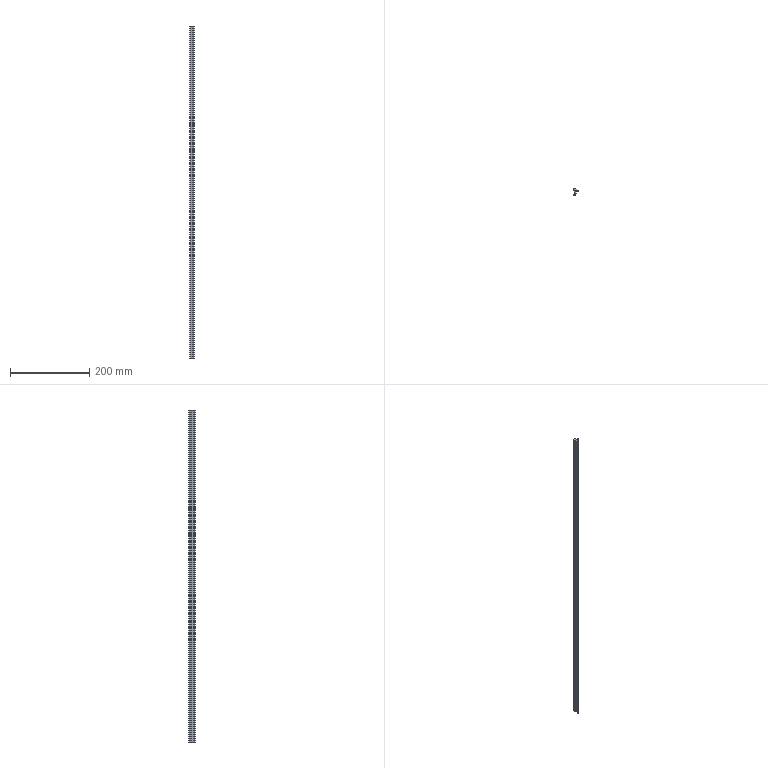Part | SolidWorks | features BaseBody 1, MoveFace 1 | 1 solid | 20 faces | box 10.8 x 17.5 x 840 mm | volume 66192 mm3 | cylinder 11 | plane 9 | commonest cylinder face diameters 1.6 x2 14 x2 0.4 x1 0.6 x1 0.8 x1 2.6 x1
STEP:
#1=CARTESIAN_POINT('',(-3.236,-11.055,740.));
#2=VERTEX_POINT('',#1);
#3=CARTESIAN_POINT('',(-4.3,-10.3,740.));
#4=VERTEX_POINT('',#3);
#5=CARTESIAN_POINT('',(-3.5,-10.3,740.));
#6=DIRECTION('',(0.,0.,-1.));
#7=DIRECTION('',(1.,0.,0.));
#8=AXIS2_PLACEMENT_3D('',#5,#6,#7);
#9=CIRCLE('',#8,0.8);
#10=EDGE_CURVE('',#2,#4,#9,.T.);
#11=ORIENTED_EDGE('',*,*,#10,.T.);
#12=CARTESIAN_POINT('',(-4.3,-10.3,-100.));
#13=VERTEX_POINT('',#12);
#14=CARTESIAN_POINT('',(-4.3,-10.3,-100.));
#15=DIRECTION('',(0.,0.,-1.));
#16=VECTOR('',#15,1000.);
#17=LINE('',#14,#16);
#18=EDGE_CURVE('',#4,#13,#17,.T.);
#19=ORIENTED_EDGE('',*,*,#18,.T.);
#20=CARTESIAN_POINT('',(-3.236,-11.055,-100.));
#21=VERTEX_POINT('',#20);
#22=CARTESIAN_POINT('',(-3.5,-10.3,-100.));
#23=DIRECTION('',(0.,0.,1.));
#24=DIRECTION('',(-1.,0.,0.));
#25=AXIS2_PLACEMENT_3D('',#22,#23,#24);
#26=CIRCLE('',#25,0.8);
#27=EDGE_CURVE('',#13,#21,#26,.T.);
#28=ORIENTED_EDGE('',*,*,#27,.T.);
#29=CARTESIAN_POINT('',(-3.236,-11.055,-100.));
#30=DIRECTION('',(0.,0.,-1.));
#31=VECTOR('',#30,1000.);
#32=LINE('',#29,#31);
#33=EDGE_CURVE('',#2,#21,#32,.T.);
#34=ORIENTED_EDGE('',*,*,#33,.F.);
#35=EDGE_LOOP('',(#11,#19,#28,#34));
#36=FACE_OUTER_BOUND('',#35,.T.);
#37=CARTESIAN_POINT('',(-3.5,-10.3,-100.));
#38=DIRECTION('',(0.,0.,-1.));
#39=DIRECTION('',(-1.,0.,0.));
#40=AXIS2_PLACEMENT_3D('',#37,#38,#39);
#41=CYLINDRICAL_SURFACE('',#40,0.8);
#42=ADVANCED_FACE('',(#36),#41,.T.);
#43=CARTESIAN_POINT('',(1.184,-6.397,-100.));
#44=VERTEX_POINT('',#43);
#45=CARTESIAN_POINT('',(-5.702,-4.29,-100.));
#46=DIRECTION('',(0.,0.,1.));
#47=DIRECTION('',(-1.,0.,0.));
#48=AXIS2_PLACEMENT_3D('',#45,#46,#47);
#49=CIRCLE('',#48,7.201);
#50=EDGE_CURVE('',#21,#44,#49,.T.);
#51=ORIENTED_EDGE('',*,*,#50,.T.);
#52=CARTESIAN_POINT('',(1.184,-6.397,740.));
#53=VERTEX_POINT('',#52);
#54=CARTESIAN_POINT('',(1.184,-6.397,-100.));
#55=DIRECTION('',(0.,0.,1.));
#56=VECTOR('',#55,1000.);
#57=LINE('',#54,#56);
#58=EDGE_CURVE('',#44,#53,#57,.T.);
#59=ORIENTED_EDGE('',*,*,#58,.T.);
#60=CARTESIAN_POINT('',(-5.702,-4.29,740.));
#61=DIRECTION('',(0.,0.,-1.));
#62=DIRECTION('',(1.,0.,0.));
#63=AXIS2_PLACEMENT_3D('',#60,#61,#62);
#64=CIRCLE('',#63,7.201);
#65=EDGE_CURVE('',#53,#2,#64,.T.);
#66=ORIENTED_EDGE('',*,*,#65,.T.);
#67=ORIENTED_EDGE('',*,*,#33,.T.);
#68=EDGE_LOOP('',(#51,#59,#66,#67));
#69=FACE_OUTER_BOUND('',#68,.T.);
#70=CARTESIAN_POINT('',(-5.702,-4.29,-100.));
#71=DIRECTION('',(0.,0.,-1.));
#72=DIRECTION('',(-1.,0.,0.));
#73=AXIS2_PLACEMENT_3D('',#70,#71,#72);
#74=CYLINDRICAL_SURFACE('',#73,7.201);
#75=ADVANCED_FACE('',(#69),#74,.T.);
#76=CARTESIAN_POINT('',(0.9,-6.,-100.));
#77=VERTEX_POINT('',#76);
#78=CARTESIAN_POINT('',(0.9,-6.3,-100.));
#79=DIRECTION('',(0.,0.,1.));
#80=DIRECTION('',(-1.,0.,0.));
#81=AXIS2_PLACEMENT_3D('',#78,#79,#80);
#82=CIRCLE('',#81,0.3);
#83=EDGE_CURVE('',#44,#77,#82,.T.);
#84=ORIENTED_EDGE('',*,*,#83,.T.);
#85=CARTESIAN_POINT('',(0.9,-6.,740.));
#86=VERTEX_POINT('',#85);
#87=CARTESIAN_POINT('',(0.9,-6.,-100.));
#88=DIRECTION('',(0.,0.,1.));
#89=VECTOR('',#88,1000.);
#90=LINE('',#87,#89);
#91=EDGE_CURVE('',#77,#86,#90,.T.);
#92=ORIENTED_EDGE('',*,*,#91,.T.);
#93=CARTESIAN_POINT('',(0.9,-6.3,740.));
#94=DIRECTION('',(0.,0.,-1.));
#95=DIRECTION('',(1.,0.,0.));
#96=AXIS2_PLACEMENT_3D('',#93,#94,#95);
#97=CIRCLE('',#96,0.3);
#98=EDGE_CURVE('',#86,#53,#97,.T.);
#99=ORIENTED_EDGE('',*,*,#98,.T.);
#100=ORIENTED_EDGE('',*,*,#58,.F.);
#101=EDGE_LOOP('',(#84,#92,#99,#100));
#102=FACE_OUTER_BOUND('',#101,.T.);
#103=CARTESIAN_POINT('',(0.9,-6.3,-100.));
#104=DIRECTION('',(0.,0.,-1.));
#105=DIRECTION('',(-1.,0.,0.));
#106=AXIS2_PLACEMENT_3D('',#103,#104,#105);
#107=CYLINDRICAL_SURFACE('',#106,0.3);
#108=ADVANCED_FACE('',(#102),#107,.T.);
#109=CARTESIAN_POINT('',(-2.5,-0.5,-100.));
#110=VERTEX_POINT('',#109);
#111=CARTESIAN_POINT('',(-2.5,-6.153,-100.));
#112=VERTEX_POINT('',#111);
#113=CARTESIAN_POINT('',(-2.5,-6.397,-100.));
#114=DIRECTION('',(0.,-1.,0.));
#115=VECTOR('',#114,1000.);
#116=LINE('',#113,#115);
#117=EDGE_CURVE('',#110,#112,#116,.T.);
#118=ORIENTED_EDGE('',*,*,#117,.F.);
#119=CARTESIAN_POINT('',(-4.2,1.695,-100.));
#120=VERTEX_POINT('',#119);
#121=CARTESIAN_POINT('',(-1.701,1.875,-100.));
#122=DIRECTION('',(0.,0.,1.));
#123=DIRECTION('',(-1.,0.,0.));
#124=AXIS2_PLACEMENT_3D('',#121,#122,#123);
#125=CIRCLE('',#124,2.506);
#126=EDGE_CURVE('',#120,#110,#125,.T.);
#127=ORIENTED_EDGE('',*,*,#126,.F.);
#128=CARTESIAN_POINT('',(-4.2,5.1,-100.));
#129=VERTEX_POINT('',#128);
#130=CARTESIAN_POINT('',(-4.2,-6.397,-100.));
#131=DIRECTION('',(0.,-1.,0.));
#132=VECTOR('',#131,1000.);
#133=LINE('',#130,#132);
#134=EDGE_CURVE('',#129,#120,#133,.T.);
#135=ORIENTED_EDGE('',*,*,#134,.F.);
#136=CARTESIAN_POINT('',(-2.892,6.4,-100.));
#137=VERTEX_POINT('',#136);
#138=CARTESIAN_POINT('',(-2.9,5.1,-100.));
#139=DIRECTION('',(0.,0.,1.));
#140=DIRECTION('',(-1.,0.,0.));
#141=AXIS2_PLACEMENT_3D('',#138,#139,#140);
#142=CIRCLE('',#141,1.3);
#143=EDGE_CURVE('',#137,#129,#142,.T.);
#144=ORIENTED_EDGE('',*,*,#143,.F.);
#145=CARTESIAN_POINT('',(0.5,5.5,-100.));
#146=VERTEX_POINT('',#145);
#147=CARTESIAN_POINT('',(-2.934,-0.5999,-100.));
#148=DIRECTION('',(0.,0.,1.));
#149=DIRECTION('',(-1.,0.,0.));
#150=AXIS2_PLACEMENT_3D('',#147,#148,#149);
#151=CIRCLE('',#150,7.);
#152=EDGE_CURVE('',#146,#137,#151,.T.);
#153=ORIENTED_EDGE('',*,*,#152,.F.);
#154=CARTESIAN_POINT('',(5.5,1.7,-100.));
#155=VERTEX_POINT('',#154);
#156=CARTESIAN_POINT('',(5.5,1.7,-100.));
#157=DIRECTION('',(-0.7962,0.6051,0.));
#158=VECTOR('',#157,1000.);
#159=LINE('',#156,#158);
#160=EDGE_CURVE('',#155,#146,#159,.T.);
#161=ORIENTED_EDGE('',*,*,#160,.F.);
#162=CARTESIAN_POINT('',(6.458,-0.2215,-100.));
#163=VERTEX_POINT('',#162);
#164=CARTESIAN_POINT('',(6.458,-0.2215,-100.));
#165=DIRECTION('',(-0.4462,0.8949,0.));
#166=VECTOR('',#165,1000.);
#167=LINE('',#164,#166);
#168=EDGE_CURVE('',#163,#155,#167,.T.);
#169=ORIENTED_EDGE('',*,*,#168,.F.);
#170=CARTESIAN_POINT('',(5.895,-0.7433,-100.));
#171=VERTEX_POINT('',#170);
#172=CARTESIAN_POINT('',(6.1,-0.4,-100.));
#173=DIRECTION('',(0.,0.,1.));
#174=DIRECTION('',(-1.,0.,0.));
#175=AXIS2_PLACEMENT_3D('',#172,#173,#174);
#176=CIRCLE('',#175,0.4);
#177=EDGE_CURVE('',#171,#163,#176,.T.);
#178=ORIENTED_EDGE('',*,*,#177,.F.);
#179=CARTESIAN_POINT('',(3.,0.,-100.));
#180=VERTEX_POINT('',#179);
#181=CARTESIAN_POINT('',(2.746,-6.995,-100.));
#182=DIRECTION('',(0.,0.,-1.));
#183=DIRECTION('',(-1.,0.,0.));
#184=AXIS2_PLACEMENT_3D('',#181,#182,#183);
#185=CIRCLE('',#184,7.);
#186=EDGE_CURVE('',#180,#171,#185,.T.);
#187=ORIENTED_EDGE('',*,*,#186,.F.);
#188=CARTESIAN_POINT('',(0.,0.,-100.));
#189=VERTEX_POINT('',#188);
#190=CARTESIAN_POINT('',(-6.814,0.,-100.));
#191=DIRECTION('',(1.,0.,0.));
#192=VECTOR('',#191,1000.);
#193=LINE('',#190,#192);
#194=EDGE_CURVE('',#189,#180,#193,.T.);
#195=ORIENTED_EDGE('',*,*,#194,.F.);
#196=CARTESIAN_POINT('',(0.,-5.8,-100.));
#197=VERTEX_POINT('',#196);
#198=CARTESIAN_POINT('',(0.,-6.397,-100.));
#199=DIRECTION('',(0.,1.,0.));
#200=VECTOR('',#199,1000.);
#201=LINE('',#198,#200);
#202=EDGE_CURVE('',#197,#189,#201,.T.);
#203=ORIENTED_EDGE('',*,*,#202,.F.);
#204=CARTESIAN_POINT('',(0.2,-6.,-100.));
#205=VERTEX_POINT('',#204);
#206=CARTESIAN_POINT('',(0.2,-5.8,-100.));
#207=DIRECTION('',(0.,0.,1.));
#208=DIRECTION('',(-1.,0.,0.));
#209=AXIS2_PLACEMENT_3D('',#206,#207,#208);
#210=CIRCLE('',#209,0.2);
#211=EDGE_CURVE('',#197,#205,#210,.T.);
#212=ORIENTED_EDGE('',*,*,#211,.T.);
#213=CARTESIAN_POINT('',(-6.814,-6.,-100.));
#214=DIRECTION('',(-1.,0.,0.));
#215=VECTOR('',#214,1000.);
#216=LINE('',#213,#215);
#217=EDGE_CURVE('',#77,#205,#216,.T.);
#218=ORIENTED_EDGE('',*,*,#217,.F.);
#219=ORIENTED_EDGE('',*,*,#83,.F.);
#220=ORIENTED_EDGE('',*,*,#50,.F.);
#221=ORIENTED_EDGE('',*,*,#27,.F.);
#222=CARTESIAN_POINT('',(-3.998,-9.674,-100.));
#223=VERTEX_POINT('',#222);
#224=CARTESIAN_POINT('',(-3.5,-10.3,-100.));
#225=DIRECTION('',(0.,0.,1.));
#226=DIRECTION('',(-1.,0.,0.));
#227=AXIS2_PLACEMENT_3D('',#224,#225,#226);
#228=CIRCLE('',#227,0.8);
#229=EDGE_CURVE('',#223,#13,#228,.T.);
#230=ORIENTED_EDGE('',*,*,#229,.F.);
#231=CARTESIAN_POINT('',(-6.814,-6.397,-100.));
#232=DIRECTION('',(0.,0.,-1.));
#233=DIRECTION('',(-1.,0.,0.));
#234=AXIS2_PLACEMENT_3D('',#231,#232,#233);
#235=CIRCLE('',#234,4.321);
#236=EDGE_CURVE('',#112,#223,#235,.T.);
#237=ORIENTED_EDGE('',*,*,#236,.F.);
#238=EDGE_LOOP('',(#118,#127,#135,#144,#153,#161,#169,#178,#187,#195,#203,#212,#218,#219,#220,#221,#230,#237));
#239=FACE_OUTER_BOUND('',#238,.T.);
#240=CARTESIAN_POINT('',(-6.814,-6.397,-100.));
#241=DIRECTION('',(0.,0.,1.));
#242=DIRECTION('',(1.,0.,0.));
#243=AXIS2_PLACEMENT_3D('',#240,#241,#242);
#244=PLANE('',#243);
#245=ADVANCED_FACE('',(#239),#244,.F.);
#246=ORIENTED_EDGE('',*,*,#18,.F.);
#247=CARTESIAN_POINT('',(-3.998,-9.674,740.));
#248=VERTEX_POINT('',#247);
#249=CARTESIAN_POINT('',(-3.5,-10.3,740.));
#250=DIRECTION('',(0.,0.,-1.));
#251=DIRECTION('',(1.,0.,0.));
#252=AXIS2_PLACEMENT_3D('',#249,#250,#251);
#253=CIRCLE('',#252,0.8);
#254=EDGE_CURVE('',#4,#248,#253,.T.);
#255=ORIENTED_EDGE('',*,*,#254,.T.);
#256=CARTESIAN_POINT('',(-3.998,-9.674,-100.));
#257=DIRECTION('',(0.,0.,-1.));
#258=VECTOR('',#257,1000.);
#259=LINE('',#256,#258);
#260=EDGE_CURVE('',#248,#223,#259,.T.);
#261=ORIENTED_EDGE('',*,*,#260,.T.);
#262=ORIENTED_EDGE('',*,*,#229,.T.);
#263=EDGE_LOOP('',(#246,#255,#261,#262));
#264=FACE_OUTER_BOUND('',#263,.T.);
#265=CARTESIAN_POINT('',(-3.5,-10.3,-100.));
#266=DIRECTION('',(0.,0.,-1.));
#267=DIRECTION('',(-1.,0.,0.));
#268=AXIS2_PLACEMENT_3D('',#265,#266,#267);
#269=CYLINDRICAL_SURFACE('',#268,0.8);
#270=ADVANCED_FACE('',(#264),#269,.T.);
#271=CARTESIAN_POINT('',(-4.2,1.695,740.));
#272=VERTEX_POINT('',#271);
#273=CARTESIAN_POINT('',(-2.5,-0.5,740.));
#274=VERTEX_POINT('',#273);
#275=CARTESIAN_POINT('',(-1.701,1.875,740.));
#276=DIRECTION('',(0.,0.,1.));
#277=DIRECTION('',(1.,0.,0.));
#278=AXIS2_PLACEMENT_3D('',#275,#276,#277);
#279=CIRCLE('',#278,2.506);
#280=EDGE_CURVE('',#272,#274,#279,.T.);
#281=ORIENTED_EDGE('',*,*,#280,.T.);
#282=CARTESIAN_POINT('',(-2.5,-6.153,740.));
#283=VERTEX_POINT('',#282);
#284=CARTESIAN_POINT('',(-2.5,-6.397,740.));
#285=DIRECTION('',(0.,-1.,0.));
#286=VECTOR('',#285,1000.);
#287=LINE('',#284,#286);
#288=EDGE_CURVE('',#274,#283,#287,.T.);
#289=ORIENTED_EDGE('',*,*,#288,.T.);
#290=CARTESIAN_POINT('',(-6.814,-6.397,740.));
#291=DIRECTION('',(0.,0.,-1.));
#292=DIRECTION('',(1.,0.,0.));
#293=AXIS2_PLACEMENT_3D('',#290,#291,#292);
#294=CIRCLE('',#293,4.321);
#295=EDGE_CURVE('',#283,#248,#294,.T.);
#296=ORIENTED_EDGE('',*,*,#295,.T.);
#297=ORIENTED_EDGE('',*,*,#254,.F.);
#298=ORIENTED_EDGE('',*,*,#10,.F.);
#299=ORIENTED_EDGE('',*,*,#65,.F.);
#300=ORIENTED_EDGE('',*,*,#98,.F.);
#301=CARTESIAN_POINT('',(0.2,-6.,740.));
#302=VERTEX_POINT('',#301);
#303=CARTESIAN_POINT('',(-6.814,-6.,740.));
#304=DIRECTION('',(-1.,0.,0.));
#305=VECTOR('',#304,1000.);
#306=LINE('',#303,#305);
#307=EDGE_CURVE('',#86,#302,#306,.T.);
#308=ORIENTED_EDGE('',*,*,#307,.T.);
#309=CARTESIAN_POINT('',(0.,-5.8,740.));
#310=VERTEX_POINT('',#309);
#311=CARTESIAN_POINT('',(0.2,-5.8,740.));
#312=DIRECTION('',(0.,0.,-1.));
#313=DIRECTION('',(1.,0.,0.));
#314=AXIS2_PLACEMENT_3D('',#311,#312,#313);
#315=CIRCLE('',#314,0.2);
#316=EDGE_CURVE('',#302,#310,#315,.T.);
#317=ORIENTED_EDGE('',*,*,#316,.T.);
#318=CARTESIAN_POINT('',(0.,0.,740.));
#319=VERTEX_POINT('',#318);
#320=CARTESIAN_POINT('',(0.,-6.397,740.));
#321=DIRECTION('',(0.,1.,0.));
#322=VECTOR('',#321,1000.);
#323=LINE('',#320,#322);
#324=EDGE_CURVE('',#310,#319,#323,.T.);
#325=ORIENTED_EDGE('',*,*,#324,.T.);
#326=CARTESIAN_POINT('',(3.,0.,740.));
#327=VERTEX_POINT('',#326);
#328=CARTESIAN_POINT('',(-6.814,0.,740.));
#329=DIRECTION('',(1.,0.,0.));
#330=VECTOR('',#329,1000.);
#331=LINE('',#328,#330);
#332=EDGE_CURVE('',#319,#327,#331,.T.);
#333=ORIENTED_EDGE('',*,*,#332,.T.);
#334=CARTESIAN_POINT('',(5.895,-0.7433,740.));
#335=VERTEX_POINT('',#334);
#336=CARTESIAN_POINT('',(2.746,-6.995,740.));
#337=DIRECTION('',(0.,0.,-1.));
#338=DIRECTION('',(1.,0.,0.));
#339=AXIS2_PLACEMENT_3D('',#336,#337,#338);
#340=CIRCLE('',#339,7.);
#341=EDGE_CURVE('',#327,#335,#340,.T.);
#342=ORIENTED_EDGE('',*,*,#341,.T.);
#343=CARTESIAN_POINT('',(6.458,-0.2215,740.));
#344=VERTEX_POINT('',#343);
#345=CARTESIAN_POINT('',(6.1,-0.4,740.));
#346=DIRECTION('',(0.,0.,-1.));
#347=DIRECTION('',(1.,0.,0.));
#348=AXIS2_PLACEMENT_3D('',#345,#346,#347);
#349=CIRCLE('',#348,0.4);
#350=EDGE_CURVE('',#344,#335,#349,.T.);
#351=ORIENTED_EDGE('',*,*,#350,.F.);
#352=CARTESIAN_POINT('',(5.5,1.7,740.));
#353=VERTEX_POINT('',#352);
#354=CARTESIAN_POINT('',(6.282,0.1323,740.));
#355=DIRECTION('',(-0.4462,0.8949,0.));
#356=VECTOR('',#355,1000.);
#357=LINE('',#354,#356);
#358=EDGE_CURVE('',#344,#353,#357,.T.);
#359=ORIENTED_EDGE('',*,*,#358,.T.);
#360=CARTESIAN_POINT('',(0.5,5.5,740.));
#361=VERTEX_POINT('',#360);
#362=CARTESIAN_POINT('',(1.595,4.668,740.));
#363=DIRECTION('',(-0.7962,0.6051,0.));
#364=VECTOR('',#363,1000.);
#365=LINE('',#362,#364);
#366=EDGE_CURVE('',#353,#361,#365,.T.);
#367=ORIENTED_EDGE('',*,*,#366,.T.);
#368=CARTESIAN_POINT('',(-2.892,6.4,740.));
#369=VERTEX_POINT('',#368);
#370=CARTESIAN_POINT('',(-2.934,-0.5999,740.));
#371=DIRECTION('',(0.,0.,1.));
#372=DIRECTION('',(1.,0.,0.));
#373=AXIS2_PLACEMENT_3D('',#370,#371,#372);
#374=CIRCLE('',#373,7.);
#375=EDGE_CURVE('',#361,#369,#374,.T.);
#376=ORIENTED_EDGE('',*,*,#375,.T.);
#377=CARTESIAN_POINT('',(-4.2,5.1,740.));
#378=VERTEX_POINT('',#377);
#379=CARTESIAN_POINT('',(-2.9,5.1,740.));
#380=DIRECTION('',(0.,0.,1.));
#381=DIRECTION('',(1.,0.,0.));
#382=AXIS2_PLACEMENT_3D('',#379,#380,#381);
#383=CIRCLE('',#382,1.3);
#384=EDGE_CURVE('',#369,#378,#383,.T.);
#385=ORIENTED_EDGE('',*,*,#384,.T.);
#386=CARTESIAN_POINT('',(-4.2,-6.397,740.));
#387=DIRECTION('',(0.,-1.,0.));
#388=VECTOR('',#387,1000.);
#389=LINE('',#386,#388);
#390=EDGE_CURVE('',#378,#272,#389,.T.);
#391=ORIENTED_EDGE('',*,*,#390,.T.);
#392=EDGE_LOOP('',(#281,#289,#296,#297,#298,#299,#300,#308,#317,#325,#333,#342,#351,#359,#367,#376,#385,#391));
#393=FACE_OUTER_BOUND('',#392,.T.);
#394=CARTESIAN_POINT('',(-6.814,-6.397,740.));
#395=DIRECTION('',(0.,0.,1.));
#396=DIRECTION('',(1.,0.,0.));
#397=AXIS2_PLACEMENT_3D('',#394,#395,#396);
#398=PLANE('',#397);
#399=ADVANCED_FACE('',(#393),#398,.T.);
#400=ORIENTED_EDGE('',*,*,#217,.T.);
#401=CARTESIAN_POINT('',(0.2,-6.,-100.));
#402=DIRECTION('',(0.,0.,1.));
#403=VECTOR('',#402,1000.);
#404=LINE('',#401,#403);
#405=EDGE_CURVE('',#205,#302,#404,.T.);
#406=ORIENTED_EDGE('',*,*,#405,.T.);
#407=ORIENTED_EDGE('',*,*,#307,.F.);
#408=ORIENTED_EDGE('',*,*,#91,.F.);
#409=EDGE_LOOP('',(#400,#406,#407,#408));
#410=FACE_OUTER_BOUND('',#409,.T.);
#411=CARTESIAN_POINT('',(0.9,-6.,-100.));
#412=DIRECTION('',(0.,1.,0.));
#413=DIRECTION('',(0.,0.,1.));
#414=AXIS2_PLACEMENT_3D('',#411,#412,#413);
#415=PLANE('',#414);
#416=ADVANCED_FACE('',(#410),#415,.T.);
#417=CARTESIAN_POINT('',(-2.5,-6.153,-100.));
#418=DIRECTION('',(0.,0.,1.));
#419=VECTOR('',#418,1000.);
#420=LINE('',#417,#419);
#421=EDGE_CURVE('',#112,#283,#420,.T.);
#422=ORIENTED_EDGE('',*,*,#421,.F.);
#423=ORIENTED_EDGE('',*,*,#236,.T.);
#424=ORIENTED_EDGE('',*,*,#260,.F.);
#425=ORIENTED_EDGE('',*,*,#295,.F.);
#426=EDGE_LOOP('',(#422,#423,#424,#425));
#427=FACE_OUTER_BOUND('',#426,.T.);
#428=CARTESIAN_POINT('',(-6.814,-6.397,-100.));
#429=DIRECTION('',(0.,0.,-1.));
#430=DIRECTION('',(-1.,0.,0.));
#431=AXIS2_PLACEMENT_3D('',#428,#429,#430);
#432=CYLINDRICAL_SURFACE('',#431,4.321);
#433=ADVANCED_FACE('',(#427),#432,.F.);
#434=ORIENTED_EDGE('',*,*,#117,.T.);
#435=ORIENTED_EDGE('',*,*,#421,.T.);
#436=ORIENTED_EDGE('',*,*,#288,.F.);
#437=CARTESIAN_POINT('',(-2.5,-0.5,-100.));
#438=DIRECTION('',(0.,0.,-1.));
#439=VECTOR('',#438,1000.);
#440=LINE('',#437,#439);
#441=EDGE_CURVE('',#274,#110,#440,.T.);
#442=ORIENTED_EDGE('',*,*,#441,.T.);
#443=EDGE_LOOP('',(#434,#435,#436,#442));
#444=FACE_OUTER_BOUND('',#443,.T.);
#445=CARTESIAN_POINT('',(-2.5,-0.5,-100.));
#446=DIRECTION('',(-1.,0.,0.));
#447=DIRECTION('',(0.,0.,1.));
#448=AXIS2_PLACEMENT_3D('',#445,#446,#447);
#449=PLANE('',#448);
#450=ADVANCED_FACE('',(#444),#449,.T.);
#451=ORIENTED_EDGE('',*,*,#126,.T.);
#452=ORIENTED_EDGE('',*,*,#441,.F.);
#453=ORIENTED_EDGE('',*,*,#280,.F.);
#454=CARTESIAN_POINT('',(-4.2,1.695,-100.));
#455=DIRECTION('',(0.,0.,-1.));
#456=VECTOR('',#455,1000.);
#457=LINE('',#454,#456);
#458=EDGE_CURVE('',#272,#120,#457,.T.);
#459=ORIENTED_EDGE('',*,*,#458,.T.);
#460=EDGE_LOOP('',(#451,#452,#453,#459));
#461=FACE_OUTER_BOUND('',#460,.T.);
#462=CARTESIAN_POINT('',(-1.701,1.875,-100.));
#463=DIRECTION('',(0.,0.,-1.));
#464=DIRECTION('',(-1.,0.,0.));
#465=AXIS2_PLACEMENT_3D('',#462,#463,#464);
#466=CYLINDRICAL_SURFACE('',#465,2.506);
#467=ADVANCED_FACE('',(#461),#466,.T.);
#468=ORIENTED_EDGE('',*,*,#134,.T.);
#469=ORIENTED_EDGE('',*,*,#458,.F.);
#470=ORIENTED_EDGE('',*,*,#390,.F.);
#471=CARTESIAN_POINT('',(-4.2,5.1,-100.));
#472=DIRECTION('',(0.,0.,-1.));
#473=VECTOR('',#472,1000.);
#474=LINE('',#471,#473);
#475=EDGE_CURVE('',#378,#129,#474,.T.);
#476=ORIENTED_EDGE('',*,*,#475,.T.);
#477=EDGE_LOOP('',(#468,#469,#470,#476));
#478=FACE_OUTER_BOUND('',#477,.T.);
#479=CARTESIAN_POINT('',(-4.2,5.1,-100.));
#480=DIRECTION('',(-1.,0.,0.));
#481=DIRECTION('',(0.,0.,1.));
#482=AXIS2_PLACEMENT_3D('',#479,#480,#481);
#483=PLANE('',#482);
#484=ADVANCED_FACE('',(#478),#483,.T.);
#485=ORIENTED_EDGE('',*,*,#143,.T.);
#486=ORIENTED_EDGE('',*,*,#475,.F.);
#487=ORIENTED_EDGE('',*,*,#384,.F.);
#488=CARTESIAN_POINT('',(-2.892,6.4,-100.));
#489=DIRECTION('',(0.,0.,-1.));
#490=VECTOR('',#489,1000.);
#491=LINE('',#488,#490);
#492=EDGE_CURVE('',#369,#137,#491,.T.);
#493=ORIENTED_EDGE('',*,*,#492,.T.);
#494=EDGE_LOOP('',(#485,#486,#487,#493));
#495=FACE_OUTER_BOUND('',#494,.T.);
#496=CARTESIAN_POINT('',(-2.9,5.1,-100.));
#497=DIRECTION('',(0.,0.,-1.));
#498=DIRECTION('',(-1.,0.,0.));
#499=AXIS2_PLACEMENT_3D('',#496,#497,#498);
#500=CYLINDRICAL_SURFACE('',#499,1.3);
#501=ADVANCED_FACE('',(#495),#500,.T.);
#502=ORIENTED_EDGE('',*,*,#152,.T.);
#503=ORIENTED_EDGE('',*,*,#492,.F.);
#504=ORIENTED_EDGE('',*,*,#375,.F.);
#505=CARTESIAN_POINT('',(0.5,5.5,-100.));
#506=DIRECTION('',(0.,0.,-1.));
#507=VECTOR('',#506,1000.);
#508=LINE('',#505,#507);
#509=EDGE_CURVE('',#361,#146,#508,.T.);
#510=ORIENTED_EDGE('',*,*,#509,.T.);
#511=EDGE_LOOP('',(#502,#503,#504,#510));
#512=FACE_OUTER_BOUND('',#511,.T.);
#513=CARTESIAN_POINT('',(-2.934,-0.5999,-100.));
#514=DIRECTION('',(0.,0.,-1.));
#515=DIRECTION('',(-1.,0.,0.));
#516=AXIS2_PLACEMENT_3D('',#513,#514,#515);
#517=CYLINDRICAL_SURFACE('',#516,7.);
#518=ADVANCED_FACE('',(#512),#517,.T.);
#519=ORIENTED_EDGE('',*,*,#160,.T.);
#520=ORIENTED_EDGE('',*,*,#509,.F.);
#521=ORIENTED_EDGE('',*,*,#366,.F.);
#522=CARTESIAN_POINT('',(5.5,1.7,-100.));
#523=DIRECTION('',(0.,0.,-1.));
#524=VECTOR('',#523,1000.);
#525=LINE('',#522,#524);
#526=EDGE_CURVE('',#353,#155,#525,.T.);
#527=ORIENTED_EDGE('',*,*,#526,.T.);
#528=EDGE_LOOP('',(#519,#520,#521,#527));
#529=FACE_OUTER_BOUND('',#528,.T.);
#530=CARTESIAN_POINT('',(5.5,1.7,-100.));
#531=DIRECTION('',(0.6051,0.7962,0.));
#532=DIRECTION('',(-0.7962,0.6051,0.));
#533=AXIS2_PLACEMENT_3D('',#530,#531,#532);
#534=PLANE('',#533);
#535=ADVANCED_FACE('',(#529),#534,.T.);
#536=ORIENTED_EDGE('',*,*,#168,.T.);
#537=ORIENTED_EDGE('',*,*,#526,.F.);
#538=ORIENTED_EDGE('',*,*,#358,.F.);
#539=CARTESIAN_POINT('',(6.458,-0.2215,-100.));
#540=DIRECTION('',(0.,0.,-1.));
#541=VECTOR('',#540,1000.);
#542=LINE('',#539,#541);
#543=EDGE_CURVE('',#344,#163,#542,.T.);
#544=ORIENTED_EDGE('',*,*,#543,.T.);
#545=EDGE_LOOP('',(#536,#537,#538,#544));
#546=FACE_OUTER_BOUND('',#545,.T.);
#547=CARTESIAN_POINT('',(6.458,-0.2215,-100.));
#548=DIRECTION('',(0.8949,0.4462,0.));
#549=DIRECTION('',(-0.4462,0.8949,0.));
#550=AXIS2_PLACEMENT_3D('',#547,#548,#549);
#551=PLANE('',#550);
#552=ADVANCED_FACE('',(#546),#551,.T.);
#553=CARTESIAN_POINT('',(3.,0.,-100.));
#554=DIRECTION('',(0.,0.,1.));
#555=VECTOR('',#554,1000.);
#556=LINE('',#553,#555);
#557=EDGE_CURVE('',#180,#327,#556,.T.);
#558=ORIENTED_EDGE('',*,*,#557,.F.);
#559=ORIENTED_EDGE('',*,*,#186,.T.);
#560=CARTESIAN_POINT('',(5.895,-0.7433,-100.));
#561=DIRECTION('',(0.,0.,-1.));
#562=VECTOR('',#561,1000.);
#563=LINE('',#560,#562);
#564=EDGE_CURVE('',#335,#171,#563,.T.);
#565=ORIENTED_EDGE('',*,*,#564,.F.);
#566=ORIENTED_EDGE('',*,*,#341,.F.);
#567=EDGE_LOOP('',(#558,#559,#565,#566));
#568=FACE_OUTER_BOUND('',#567,.T.);
#569=CARTESIAN_POINT('',(2.746,-6.995,-100.));
#570=DIRECTION('',(0.,0.,-1.));
#571=DIRECTION('',(-1.,0.,0.));
#572=AXIS2_PLACEMENT_3D('',#569,#570,#571);
#573=CYLINDRICAL_SURFACE('',#572,7.);
#574=ADVANCED_FACE('',(#568),#573,.F.);
#575=ORIENTED_EDGE('',*,*,#194,.T.);
#576=ORIENTED_EDGE('',*,*,#557,.T.);
#577=ORIENTED_EDGE('',*,*,#332,.F.);
#578=CARTESIAN_POINT('',(0.,0.,-100.));
#579=DIRECTION('',(0.,0.,-1.));
#580=VECTOR('',#579,1000.);
#581=LINE('',#578,#580);
#582=EDGE_CURVE('',#319,#189,#581,.T.);
#583=ORIENTED_EDGE('',*,*,#582,.T.);
#584=EDGE_LOOP('',(#575,#576,#577,#583));
#585=FACE_OUTER_BOUND('',#584,.T.);
#586=CARTESIAN_POINT('',(0.,0.,-100.));
#587=DIRECTION('',(0.,-1.,0.));
#588=DIRECTION('',(0.,0.,-1.));
#589=AXIS2_PLACEMENT_3D('',#586,#587,#588);
#590=PLANE('',#589);
#591=ADVANCED_FACE('',(#585),#590,.T.);
#592=ORIENTED_EDGE('',*,*,#202,.T.);
#593=ORIENTED_EDGE('',*,*,#582,.F.);
#594=ORIENTED_EDGE('',*,*,#324,.F.);
#595=CARTESIAN_POINT('',(0.,-5.8,-100.));
#596=DIRECTION('',(0.,0.,-1.));
#597=VECTOR('',#596,1000.);
#598=LINE('',#595,#597);
#599=EDGE_CURVE('',#310,#197,#598,.T.);
#600=ORIENTED_EDGE('',*,*,#599,.T.);
#601=EDGE_LOOP('',(#592,#593,#594,#600));
#602=FACE_OUTER_BOUND('',#601,.T.);
#603=CARTESIAN_POINT('',(0.,-5.8,-100.));
#604=DIRECTION('',(1.,0.,0.));
#605=DIRECTION('',(0.,0.,-1.));
#606=AXIS2_PLACEMENT_3D('',#603,#604,#605);
#607=PLANE('',#606);
#608=ADVANCED_FACE('',(#602),#607,.T.);
#609=ORIENTED_EDGE('',*,*,#405,.F.);
#610=ORIENTED_EDGE('',*,*,#211,.F.);
#611=ORIENTED_EDGE('',*,*,#599,.F.);
#612=ORIENTED_EDGE('',*,*,#316,.F.);
#613=EDGE_LOOP('',(#609,#610,#611,#612));
#614=FACE_OUTER_BOUND('',#613,.T.);
#615=CARTESIAN_POINT('',(0.2,-5.8,-100.));
#616=DIRECTION('',(0.,0.,-1.));
#617=DIRECTION('',(-1.,0.,0.));
#618=AXIS2_PLACEMENT_3D('',#615,#616,#617);
#619=CYLINDRICAL_SURFACE('',#618,0.2);
#620=ADVANCED_FACE('',(#614),#619,.F.);
#621=ORIENTED_EDGE('',*,*,#177,.T.);
#622=ORIENTED_EDGE('',*,*,#543,.F.);
#623=ORIENTED_EDGE('',*,*,#350,.T.);
#624=ORIENTED_EDGE('',*,*,#564,.T.);
#625=EDGE_LOOP('',(#621,#622,#623,#624));
#626=FACE_OUTER_BOUND('',#625,.T.);
#627=CARTESIAN_POINT('',(6.1,-0.4,-100.));
#628=DIRECTION('',(0.,0.,-1.));
#629=DIRECTION('',(-1.,0.,0.));
#630=AXIS2_PLACEMENT_3D('',#627,#628,#629);
#631=CYLINDRICAL_SURFACE('',#630,0.4);
#632=ADVANCED_FACE('',(#626),#631,.T.);
#633=CLOSED_SHELL('',(#42,#75,#108,#245,#270,#399,#416,#433,#450,#467,#484,#501,#518,#535,#552,#574,#591,#608,#620,#632));
#634=MANIFOLD_SOLID_BREP('',#633);
#635=CARTESIAN_POINT('',(0.,0.,0.));
#636=DIRECTION('',(0.,0.,1.));
#637=DIRECTION('',(1.,0.,0.));
#638=AXIS2_PLACEMENT_3D('',#635,#636,#637);
#639=(LENGTH_UNIT()NAMED_UNIT(*)SI_UNIT(.MILLI.,.METRE.));
#640=UNCERTAINTY_MEASURE_WITH_UNIT(LENGTH_MEASURE(0.00001),#639,'','');
#641=(NAMED_UNIT(*)PLANE_ANGLE_UNIT()SI_UNIT($,.RADIAN.));
#642=(NAMED_UNIT(*)SI_UNIT($,.STERADIAN.)SOLID_ANGLE_UNIT());
#643=(GEOMETRIC_REPRESENTATION_CONTEXT(3)GLOBAL_UNCERTAINTY_ASSIGNED_CONTEXT((#640))GLOBAL_UNIT_ASSIGNED_CONTEXT((#639,#641,#642))REPRESENTATION_CONTEXT('',''));
#644=ADVANCED_BREP_SHAPE_REPRESENTATION('',(#634,#638),#643);